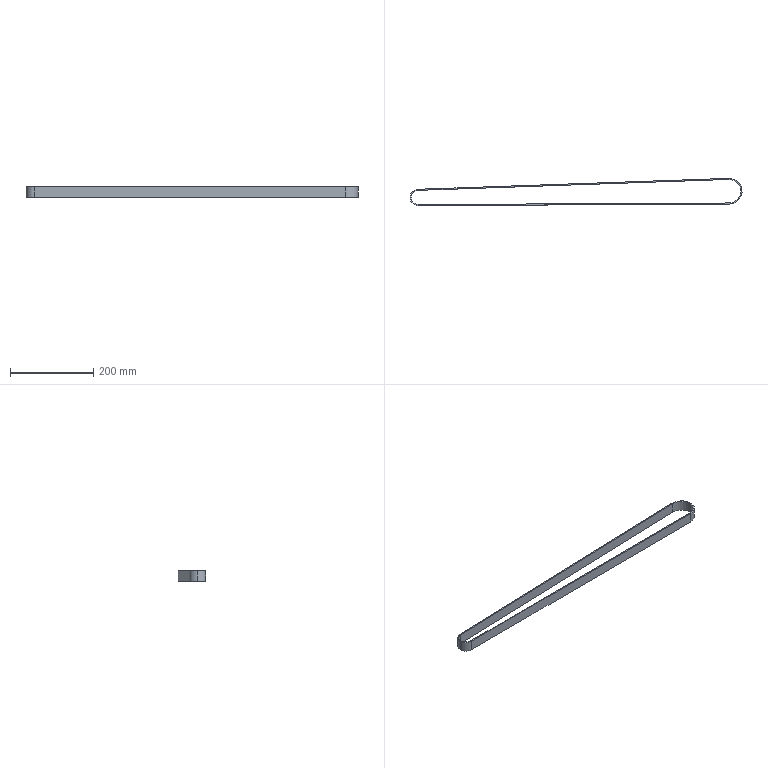Part | STEP file | Belt 4-1^ traction group | 1 solid | 12 faces | box 796.315 x 65.431 x 25 mm | volume 107582 mm3 | cylinder 6 | plane 6 | commonest cylinder face diameters 34 x2 39.24 x2 56.45 x1 61.69 x1
STEP:
#1=CARTESIAN_POINT('',(0.,0.,0.));
#2=DIRECTION('',(0.,0.,1.));
#3=DIRECTION('',(1.,0.,0.));
#4=AXIS2_PLACEMENT_3D('',#1,#2,#3);
#5=CARTESIAN_POINT('',(-0.5968,16.99,25.));
#6=VERTEX_POINT('',#5);
#7=CARTESIAN_POINT('',(-0.5968,16.99,0.));
#8=VERTEX_POINT('',#7);
#9=CARTESIAN_POINT('',(-0.5968,16.99,25.));
#10=DIRECTION('',(0.,0.,-1.));
#11=VECTOR('',#10,1.);
#12=LINE('',#9,#11);
#13=CARTESIAN_POINT('',(0.,0.,25.));
#14=DIRECTION('',(0.,0.,-1.));
#15=DIRECTION('',(-1.,0.,0.));
#16=AXIS2_PLACEMENT_3D('',#13,#14,#15);
#17=CYLINDRICAL_SURFACE('',#16,17.);
#18=CARTESIAN_POINT('',(1.536,0.));
#19=DIRECTION('',(0.,1.));
#20=VECTOR('',#19,1.);
#21=LINE('',#18,#20);
#22=(GEOMETRIC_REPRESENTATION_CONTEXT(2)PARAMETRIC_REPRESENTATION_CONTEXT()REPRESENTATION_CONTEXT('',''));
#23=DEFINITIONAL_REPRESENTATION('',(#21),#22);
#24=PCURVE('',#17,#23);
#25=CARTESIAN_POINT('',(744.859,43.174,25.));
#26=DIRECTION('',(0.0351,-0.9994,0.));
#27=DIRECTION('',(0.9994,0.0351,0.));
#28=AXIS2_PLACEMENT_3D('',#25,#26,#27);
#29=PLANE('',#28);
#30=CARTESIAN_POINT('',(-745.916,0.));
#31=DIRECTION('',(0.,-1.));
#32=VECTOR('',#31,1.);
#33=LINE('',#30,#32);
#34=(GEOMETRIC_REPRESENTATION_CONTEXT(2)PARAMETRIC_REPRESENTATION_CONTEXT()REPRESENTATION_CONTEXT('',''));
#35=DEFINITIONAL_REPRESENTATION('',(#33),#34);
#36=PCURVE('',#29,#35);
#37=SURFACE_CURVE('',#12,(#24,#36),.PCURVE_S1.);
#38=EDGE_CURVE('',#6,#8,#37,.T.);
#39=ORIENTED_EDGE('',*,*,#38,.T.);
#40=CARTESIAN_POINT('',(-17.,0.,0.));
#41=VERTEX_POINT('',#40);
#42=CARTESIAN_POINT('',(0.,0.,0.));
#43=DIRECTION('',(0.,0.,1.));
#44=DIRECTION('',(1.,0.,0.));
#45=AXIS2_PLACEMENT_3D('',#42,#43,#44);
#46=CIRCLE('',#45,17.);
#47=CARTESIAN_POINT('',(3.142,25.));
#48=DIRECTION('',(-1.,0.));
#49=VECTOR('',#48,1.);
#50=LINE('',#47,#49);
#51=(GEOMETRIC_REPRESENTATION_CONTEXT(2)PARAMETRIC_REPRESENTATION_CONTEXT()REPRESENTATION_CONTEXT('',''));
#52=DEFINITIONAL_REPRESENTATION('',(#50),#51);
#53=PCURVE('',#17,#52);
#54=CARTESIAN_POINT('',(745.85,14.966,0.));
#55=DIRECTION('',(0.,0.,1.));
#56=DIRECTION('',(1.,0.,0.));
#57=AXIS2_PLACEMENT_3D('',#54,#55,#56);
#58=PLANE('',#57);
#59=CARTESIAN_POINT('',(-745.85,-14.966));
#60=DIRECTION('',(1.,0.));
#61=AXIS2_PLACEMENT_2D('',#59,#60);
#62=CIRCLE('',#61,17.);
#63=(GEOMETRIC_REPRESENTATION_CONTEXT(2)PARAMETRIC_REPRESENTATION_CONTEXT()REPRESENTATION_CONTEXT('',''));
#64=DEFINITIONAL_REPRESENTATION('',(#62),#63);
#65=PCURVE('',#58,#64);
#66=SURFACE_CURVE('',#46,(#53,#65),.PCURVE_S1.);
#67=EDGE_CURVE('',#8,#41,#66,.T.);
#68=ORIENTED_EDGE('',*,*,#67,.T.);
#69=CARTESIAN_POINT('',(-17.,0.,25.));
#70=VERTEX_POINT('',#69);
#71=CARTESIAN_POINT('',(-17.,0.,25.));
#72=DIRECTION('',(0.,0.,-1.));
#73=VECTOR('',#72,1.);
#74=LINE('',#71,#73);
#75=CARTESIAN_POINT('',(0.,0.));
#76=DIRECTION('',(0.,1.));
#77=VECTOR('',#76,1.);
#78=LINE('',#75,#77);
#79=(GEOMETRIC_REPRESENTATION_CONTEXT(2)PARAMETRIC_REPRESENTATION_CONTEXT()REPRESENTATION_CONTEXT('',''));
#80=DEFINITIONAL_REPRESENTATION('',(#78),#79);
#81=PCURVE('',#17,#80);
#82=CARTESIAN_POINT('',(0.,0.,25.));
#83=DIRECTION('',(0.,0.,-1.));
#84=DIRECTION('',(-1.,0.,0.));
#85=AXIS2_PLACEMENT_3D('',#82,#83,#84);
#86=CYLINDRICAL_SURFACE('',#85,17.);
#87=CARTESIAN_POINT('',(6.283,0.));
#88=DIRECTION('',(0.,1.));
#89=VECTOR('',#88,1.);
#90=LINE('',#87,#89);
#91=(GEOMETRIC_REPRESENTATION_CONTEXT(2)PARAMETRIC_REPRESENTATION_CONTEXT()REPRESENTATION_CONTEXT('',''));
#92=DEFINITIONAL_REPRESENTATION('',(#90),#91);
#93=PCURVE('',#86,#92);
#94=SURFACE_CURVE('',#74,(#81,#93),.PCURVE_S1.);
#95=EDGE_CURVE('',#70,#41,#94,.T.);
#96=ORIENTED_EDGE('',*,*,#95,.F.);
#97=CARTESIAN_POINT('',(0.,0.,25.));
#98=DIRECTION('',(0.,0.,1.));
#99=DIRECTION('',(1.,0.,0.));
#100=AXIS2_PLACEMENT_3D('',#97,#98,#99);
#101=CIRCLE('',#100,17.);
#102=CARTESIAN_POINT('',(3.142,0.));
#103=DIRECTION('',(-1.,0.));
#104=VECTOR('',#103,1.);
#105=LINE('',#102,#104);
#106=(GEOMETRIC_REPRESENTATION_CONTEXT(2)PARAMETRIC_REPRESENTATION_CONTEXT()REPRESENTATION_CONTEXT('',''));
#107=DEFINITIONAL_REPRESENTATION('',(#105),#106);
#108=PCURVE('',#17,#107);
#109=CARTESIAN_POINT('',(745.85,14.966,25.));
#110=DIRECTION('',(0.,0.,1.));
#111=DIRECTION('',(1.,0.,0.));
#112=AXIS2_PLACEMENT_3D('',#109,#110,#111);
#113=PLANE('',#112);
#114=CARTESIAN_POINT('',(-745.85,-14.966));
#115=DIRECTION('',(1.,0.));
#116=AXIS2_PLACEMENT_2D('',#114,#115);
#117=CIRCLE('',#116,17.);
#118=(GEOMETRIC_REPRESENTATION_CONTEXT(2)PARAMETRIC_REPRESENTATION_CONTEXT()REPRESENTATION_CONTEXT('',''));
#119=DEFINITIONAL_REPRESENTATION('',(#117),#118);
#120=PCURVE('',#113,#119);
#121=SURFACE_CURVE('',#101,(#108,#120),.PCURVE_S1.);
#122=EDGE_CURVE('',#6,#70,#121,.T.);
#123=ORIENTED_EDGE('',*,*,#122,.F.);
#124=EDGE_LOOP('',(#39,#68,#96,#123));
#125=FACE_BOUND('',#124,.F.);
#126=ADVANCED_FACE('',(#125),#17,.F.);
#127=CARTESIAN_POINT('',(-19.62,0.,25.));
#128=VERTEX_POINT('',#127);
#129=CARTESIAN_POINT('',(0.09841,-19.62,25.));
#130=VERTEX_POINT('',#129);
#131=CARTESIAN_POINT('',(0.,0.,25.));
#132=DIRECTION('',(0.,0.,1.));
#133=DIRECTION('',(1.,0.,0.));
#134=AXIS2_PLACEMENT_3D('',#131,#132,#133);
#135=CIRCLE('',#134,19.62);
#136=CARTESIAN_POINT('',(0.,0.,25.));
#137=DIRECTION('',(0.,0.,-1.));
#138=DIRECTION('',(-1.,0.,0.));
#139=AXIS2_PLACEMENT_3D('',#136,#137,#138);
#140=CYLINDRICAL_SURFACE('',#139,19.62);
#141=CARTESIAN_POINT('',(9.425,0.));
#142=DIRECTION('',(-1.,0.));
#143=VECTOR('',#142,1.);
#144=LINE('',#141,#143);
#145=(GEOMETRIC_REPRESENTATION_CONTEXT(2)PARAMETRIC_REPRESENTATION_CONTEXT()REPRESENTATION_CONTEXT('',''));
#146=DEFINITIONAL_REPRESENTATION('',(#144),#145);
#147=PCURVE('',#140,#146);
#148=CARTESIAN_POINT('',(-745.85,-14.966));
#149=DIRECTION('',(1.,0.));
#150=AXIS2_PLACEMENT_2D('',#148,#149);
#151=CIRCLE('',#150,19.62);
#152=(GEOMETRIC_REPRESENTATION_CONTEXT(2)PARAMETRIC_REPRESENTATION_CONTEXT()REPRESENTATION_CONTEXT('',''));
#153=DEFINITIONAL_REPRESENTATION('',(#151),#152);
#154=PCURVE('',#113,#153);
#155=SURFACE_CURVE('',#135,(#147,#154),.PCURVE_S1.);
#156=EDGE_CURVE('',#128,#130,#155,.T.);
#157=ORIENTED_EDGE('',*,*,#156,.F.);
#158=CARTESIAN_POINT('',(-19.62,0.,0.));
#159=VERTEX_POINT('',#158);
#160=CARTESIAN_POINT('',(-19.62,0.,25.));
#161=DIRECTION('',(0.,0.,-1.));
#162=VECTOR('',#161,1.);
#163=LINE('',#160,#162);
#164=CARTESIAN_POINT('',(6.283,0.));
#165=DIRECTION('',(0.,1.));
#166=VECTOR('',#165,1.);
#167=LINE('',#164,#166);
#168=(GEOMETRIC_REPRESENTATION_CONTEXT(2)PARAMETRIC_REPRESENTATION_CONTEXT()REPRESENTATION_CONTEXT('',''));
#169=DEFINITIONAL_REPRESENTATION('',(#167),#168);
#170=PCURVE('',#140,#169);
#171=CARTESIAN_POINT('',(0.,0.,25.));
#172=DIRECTION('',(0.,0.,-1.));
#173=DIRECTION('',(-1.,0.,0.));
#174=AXIS2_PLACEMENT_3D('',#171,#172,#173);
#175=CYLINDRICAL_SURFACE('',#174,19.62);
#176=CARTESIAN_POINT('',(0.,0.));
#177=DIRECTION('',(0.,1.));
#178=VECTOR('',#177,1.);
#179=LINE('',#176,#178);
#180=(GEOMETRIC_REPRESENTATION_CONTEXT(2)PARAMETRIC_REPRESENTATION_CONTEXT()REPRESENTATION_CONTEXT('',''));
#181=DEFINITIONAL_REPRESENTATION('',(#179),#180);
#182=PCURVE('',#175,#181);
#183=SURFACE_CURVE('',#163,(#170,#182),.PCURVE_S1.);
#184=EDGE_CURVE('',#128,#159,#183,.T.);
#185=ORIENTED_EDGE('',*,*,#184,.T.);
#186=CARTESIAN_POINT('',(0.09841,-19.62,0.));
#187=VERTEX_POINT('',#186);
#188=CARTESIAN_POINT('',(0.,0.,0.));
#189=DIRECTION('',(0.,0.,1.));
#190=DIRECTION('',(1.,0.,0.));
#191=AXIS2_PLACEMENT_3D('',#188,#189,#190);
#192=CIRCLE('',#191,19.62);
#193=CARTESIAN_POINT('',(9.425,25.));
#194=DIRECTION('',(-1.,0.));
#195=VECTOR('',#194,1.);
#196=LINE('',#193,#195);
#197=(GEOMETRIC_REPRESENTATION_CONTEXT(2)PARAMETRIC_REPRESENTATION_CONTEXT()REPRESENTATION_CONTEXT('',''));
#198=DEFINITIONAL_REPRESENTATION('',(#196),#197);
#199=PCURVE('',#140,#198);
#200=CARTESIAN_POINT('',(-745.85,-14.966));
#201=DIRECTION('',(1.,0.));
#202=AXIS2_PLACEMENT_2D('',#200,#201);
#203=CIRCLE('',#202,19.62);
#204=(GEOMETRIC_REPRESENTATION_CONTEXT(2)PARAMETRIC_REPRESENTATION_CONTEXT()REPRESENTATION_CONTEXT('',''));
#205=DEFINITIONAL_REPRESENTATION('',(#203),#204);
#206=PCURVE('',#58,#205);
#207=SURFACE_CURVE('',#192,(#199,#206),.PCURVE_S1.);
#208=EDGE_CURVE('',#159,#187,#207,.T.);
#209=ORIENTED_EDGE('',*,*,#208,.T.);
#210=CARTESIAN_POINT('',(0.09841,-19.62,25.));
#211=DIRECTION('',(0.,0.,-1.));
#212=VECTOR('',#211,1.);
#213=LINE('',#210,#212);
#214=CARTESIAN_POINT('',(4.707,0.));
#215=DIRECTION('',(0.,1.));
#216=VECTOR('',#215,1.);
#217=LINE('',#214,#216);
#218=(GEOMETRIC_REPRESENTATION_CONTEXT(2)PARAMETRIC_REPRESENTATION_CONTEXT()REPRESENTATION_CONTEXT('',''));
#219=DEFINITIONAL_REPRESENTATION('',(#217),#218);
#220=PCURVE('',#140,#219);
#221=CARTESIAN_POINT('',(0.09841,-19.62,25.));
#222=DIRECTION('',(-0.005016,1.,0.));
#223=DIRECTION('',(-1.,-0.005016,0.));
#224=AXIS2_PLACEMENT_3D('',#221,#222,#223);
#225=PLANE('',#224);
#226=CARTESIAN_POINT('',(0.,0.));
#227=DIRECTION('',(0.,-1.));
#228=VECTOR('',#227,1.);
#229=LINE('',#226,#228);
#230=(GEOMETRIC_REPRESENTATION_CONTEXT(2)PARAMETRIC_REPRESENTATION_CONTEXT()REPRESENTATION_CONTEXT('',''));
#231=DEFINITIONAL_REPRESENTATION('',(#229),#230);
#232=PCURVE('',#225,#231);
#233=SURFACE_CURVE('',#213,(#220,#232),.PCURVE_S1.);
#234=EDGE_CURVE('',#130,#187,#233,.T.);
#235=ORIENTED_EDGE('',*,*,#234,.F.);
#236=EDGE_LOOP('',(#157,#185,#209,#235));
#237=FACE_BOUND('',#236,.T.);
#238=ADVANCED_FACE('',(#237),#140,.T.);
#239=CARTESIAN_POINT('',(746.005,-15.878,25.));
#240=VERTEX_POINT('',#239);
#241=CARTESIAN_POINT('',(744.767,45.792,25.));
#242=VERTEX_POINT('',#241);
#243=CARTESIAN_POINT('',(745.85,14.966,25.));
#244=DIRECTION('',(0.,0.,1.));
#245=DIRECTION('',(1.,0.,0.));
#246=AXIS2_PLACEMENT_3D('',#243,#244,#245);
#247=CIRCLE('',#246,30.845);
#248=CARTESIAN_POINT('',(0.,0.));
#249=DIRECTION('',(1.,0.));
#250=AXIS2_PLACEMENT_2D('',#248,#249);
#251=CIRCLE('',#250,30.845);
#252=(GEOMETRIC_REPRESENTATION_CONTEXT(2)PARAMETRIC_REPRESENTATION_CONTEXT()REPRESENTATION_CONTEXT('',''));
#253=DEFINITIONAL_REPRESENTATION('',(#251),#252);
#254=PCURVE('',#113,#253);
#255=CARTESIAN_POINT('',(745.85,14.966,25.));
#256=DIRECTION('',(0.,0.,-1.));
#257=DIRECTION('',(-1.,0.,0.));
#258=AXIS2_PLACEMENT_3D('',#255,#256,#257);
#259=CYLINDRICAL_SURFACE('',#258,30.845);
#260=CARTESIAN_POINT('',(9.425,0.));
#261=DIRECTION('',(-1.,0.));
#262=VECTOR('',#261,1.);
#263=LINE('',#260,#262);
#264=(GEOMETRIC_REPRESENTATION_CONTEXT(2)PARAMETRIC_REPRESENTATION_CONTEXT()REPRESENTATION_CONTEXT('',''));
#265=DEFINITIONAL_REPRESENTATION('',(#263),#264);
#266=PCURVE('',#259,#265);
#267=SURFACE_CURVE('',#247,(#254,#266),.PCURVE_S1.);
#268=EDGE_CURVE('',#240,#242,#267,.T.);
#269=ORIENTED_EDGE('',*,*,#268,.T.);
#270=CARTESIAN_POINT('',(-0.6887,19.608,25.));
#271=VERTEX_POINT('',#270);
#272=CARTESIAN_POINT('',(744.767,45.792,25.));
#273=DIRECTION('',(-0.9994,-0.0351,0.));
#274=VECTOR('',#273,1.);
#275=LINE('',#272,#274);
#276=CARTESIAN_POINT('',(-1.083,30.826));
#277=DIRECTION('',(-0.9994,-0.0351));
#278=VECTOR('',#277,1.);
#279=LINE('',#276,#278);
#280=(GEOMETRIC_REPRESENTATION_CONTEXT(2)PARAMETRIC_REPRESENTATION_CONTEXT()REPRESENTATION_CONTEXT('',''));
#281=DEFINITIONAL_REPRESENTATION('',(#279),#280);
#282=PCURVE('',#113,#281);
#283=CARTESIAN_POINT('',(744.767,45.792,25.));
#284=DIRECTION('',(0.0351,-0.9994,0.));
#285=DIRECTION('',(0.9994,0.0351,0.));
#286=AXIS2_PLACEMENT_3D('',#283,#284,#285);
#287=PLANE('',#286);
#288=CARTESIAN_POINT('',(0.,0.));
#289=DIRECTION('',(-1.,0.));
#290=VECTOR('',#289,1.);
#291=LINE('',#288,#290);
#292=(GEOMETRIC_REPRESENTATION_CONTEXT(2)PARAMETRIC_REPRESENTATION_CONTEXT()REPRESENTATION_CONTEXT('',''));
#293=DEFINITIONAL_REPRESENTATION('',(#291),#292);
#294=PCURVE('',#287,#293);
#295=SURFACE_CURVE('',#275,(#282,#294),.PCURVE_S1.);
#296=EDGE_CURVE('',#242,#271,#295,.T.);
#297=ORIENTED_EDGE('',*,*,#296,.T.);
#298=CARTESIAN_POINT('',(0.,0.,25.));
#299=DIRECTION('',(0.,0.,1.));
#300=DIRECTION('',(1.,0.,0.));
#301=AXIS2_PLACEMENT_3D('',#298,#299,#300);
#302=CIRCLE('',#301,19.62);
#303=CARTESIAN_POINT('',(-745.85,-14.966));
#304=DIRECTION('',(1.,0.));
#305=AXIS2_PLACEMENT_2D('',#303,#304);
#306=CIRCLE('',#305,19.62);
#307=(GEOMETRIC_REPRESENTATION_CONTEXT(2)PARAMETRIC_REPRESENTATION_CONTEXT()REPRESENTATION_CONTEXT('',''));
#308=DEFINITIONAL_REPRESENTATION('',(#306),#307);
#309=PCURVE('',#113,#308);
#310=CARTESIAN_POINT('',(3.142,0.));
#311=DIRECTION('',(-1.,0.));
#312=VECTOR('',#311,1.);
#313=LINE('',#310,#312);
#314=(GEOMETRIC_REPRESENTATION_CONTEXT(2)PARAMETRIC_REPRESENTATION_CONTEXT()REPRESENTATION_CONTEXT('',''));
#315=DEFINITIONAL_REPRESENTATION('',(#313),#314);
#316=PCURVE('',#175,#315);
#317=SURFACE_CURVE('',#302,(#309,#316),.PCURVE_S1.);
#318=EDGE_CURVE('',#271,#128,#317,.T.);
#319=ORIENTED_EDGE('',*,*,#318,.T.);
#320=ORIENTED_EDGE('',*,*,#156,.T.);
#321=CARTESIAN_POINT('',(0.09841,-19.62,25.));
#322=DIRECTION('',(1.,0.005016,0.));
#323=VECTOR('',#322,1.);
#324=LINE('',#321,#323);
#325=CARTESIAN_POINT('',(-745.751,-34.586));
#326=DIRECTION('',(1.,0.005016));
#327=VECTOR('',#326,1.);
#328=LINE('',#325,#327);
#329=(GEOMETRIC_REPRESENTATION_CONTEXT(2)PARAMETRIC_REPRESENTATION_CONTEXT()REPRESENTATION_CONTEXT('',''));
#330=DEFINITIONAL_REPRESENTATION('',(#328),#329);
#331=PCURVE('',#113,#330);
#332=CARTESIAN_POINT('',(0.,0.));
#333=DIRECTION('',(-1.,0.));
#334=VECTOR('',#333,1.);
#335=LINE('',#332,#334);
#336=(GEOMETRIC_REPRESENTATION_CONTEXT(2)PARAMETRIC_REPRESENTATION_CONTEXT()REPRESENTATION_CONTEXT('',''));
#337=DEFINITIONAL_REPRESENTATION('',(#335),#336);
#338=PCURVE('',#225,#337);
#339=SURFACE_CURVE('',#324,(#331,#338),.PCURVE_S1.);
#340=EDGE_CURVE('',#130,#240,#339,.T.);
#341=ORIENTED_EDGE('',*,*,#340,.T.);
#342=EDGE_LOOP('',(#269,#297,#319,#320,#341));
#343=FACE_BOUND('',#342,.T.);
#344=CARTESIAN_POINT('',(744.859,43.174,25.));
#345=VERTEX_POINT('',#344);
#346=CARTESIAN_POINT('',(744.859,43.174,25.));
#347=DIRECTION('',(-0.9994,-0.0351,0.));
#348=VECTOR('',#347,1.);
#349=LINE('',#346,#348);
#350=CARTESIAN_POINT('',(-0.9908,28.208));
#351=DIRECTION('',(-0.9994,-0.0351));
#352=VECTOR('',#351,1.);
#353=LINE('',#350,#352);
#354=(GEOMETRIC_REPRESENTATION_CONTEXT(2)PARAMETRIC_REPRESENTATION_CONTEXT()REPRESENTATION_CONTEXT('',''));
#355=DEFINITIONAL_REPRESENTATION('',(#353),#354);
#356=PCURVE('',#113,#355);
#357=CARTESIAN_POINT('',(0.,0.));
#358=DIRECTION('',(-1.,0.));
#359=VECTOR('',#358,1.);
#360=LINE('',#357,#359);
#361=(GEOMETRIC_REPRESENTATION_CONTEXT(2)PARAMETRIC_REPRESENTATION_CONTEXT()REPRESENTATION_CONTEXT('',''));
#362=DEFINITIONAL_REPRESENTATION('',(#360),#361);
#363=PCURVE('',#29,#362);
#364=SURFACE_CURVE('',#349,(#356,#363),.PCURVE_S1.);
#365=EDGE_CURVE('',#345,#6,#364,.T.);
#366=ORIENTED_EDGE('',*,*,#365,.F.);
#367=CARTESIAN_POINT('',(745.991,-13.258,25.));
#368=VERTEX_POINT('',#367);
#369=CARTESIAN_POINT('',(745.85,14.966,25.));
#370=DIRECTION('',(0.,0.,1.));
#371=DIRECTION('',(1.,0.,0.));
#372=AXIS2_PLACEMENT_3D('',#369,#370,#371);
#373=CIRCLE('',#372,28.225);
#374=CARTESIAN_POINT('',(0.,0.));
#375=DIRECTION('',(1.,0.));
#376=AXIS2_PLACEMENT_2D('',#374,#375);
#377=CIRCLE('',#376,28.225);
#378=(GEOMETRIC_REPRESENTATION_CONTEXT(2)PARAMETRIC_REPRESENTATION_CONTEXT()REPRESENTATION_CONTEXT('',''));
#379=DEFINITIONAL_REPRESENTATION('',(#377),#378);
#380=PCURVE('',#113,#379);
#381=CARTESIAN_POINT('',(745.85,14.966,25.));
#382=DIRECTION('',(0.,0.,-1.));
#383=DIRECTION('',(-1.,0.,0.));
#384=AXIS2_PLACEMENT_3D('',#381,#382,#383);
#385=CYLINDRICAL_SURFACE('',#384,28.225);
#386=CARTESIAN_POINT('',(9.425,0.));
#387=DIRECTION('',(-1.,0.));
#388=VECTOR('',#387,1.);
#389=LINE('',#386,#388);
#390=(GEOMETRIC_REPRESENTATION_CONTEXT(2)PARAMETRIC_REPRESENTATION_CONTEXT()REPRESENTATION_CONTEXT('',''));
#391=DEFINITIONAL_REPRESENTATION('',(#389),#390);
#392=PCURVE('',#385,#391);
#393=SURFACE_CURVE('',#373,(#380,#392),.PCURVE_S1.);
#394=EDGE_CURVE('',#368,#345,#393,.T.);
#395=ORIENTED_EDGE('',*,*,#394,.F.);
#396=CARTESIAN_POINT('',(0.08527,-17.,25.));
#397=VERTEX_POINT('',#396);
#398=CARTESIAN_POINT('',(0.08527,-17.,25.));
#399=DIRECTION('',(1.,0.005016,0.));
#400=VECTOR('',#399,1.);
#401=LINE('',#398,#400);
#402=CARTESIAN_POINT('',(-745.765,-31.966));
#403=DIRECTION('',(1.,0.005016));
#404=VECTOR('',#403,1.);
#405=LINE('',#402,#404);
#406=(GEOMETRIC_REPRESENTATION_CONTEXT(2)PARAMETRIC_REPRESENTATION_CONTEXT()REPRESENTATION_CONTEXT('',''));
#407=DEFINITIONAL_REPRESENTATION('',(#405),#406);
#408=PCURVE('',#113,#407);
#409=CARTESIAN_POINT('',(0.08527,-17.,25.));
#410=DIRECTION('',(-0.005016,1.,0.));
#411=DIRECTION('',(-1.,-0.005016,0.));
#412=AXIS2_PLACEMENT_3D('',#409,#410,#411);
#413=PLANE('',#412);
#414=CARTESIAN_POINT('',(0.,0.));
#415=DIRECTION('',(-1.,0.));
#416=VECTOR('',#415,1.);
#417=LINE('',#414,#416);
#418=(GEOMETRIC_REPRESENTATION_CONTEXT(2)PARAMETRIC_REPRESENTATION_CONTEXT()REPRESENTATION_CONTEXT('',''));
#419=DEFINITIONAL_REPRESENTATION('',(#417),#418);
#420=PCURVE('',#413,#419);
#421=SURFACE_CURVE('',#401,(#408,#420),.PCURVE_S1.);
#422=EDGE_CURVE('',#397,#368,#421,.T.);
#423=ORIENTED_EDGE('',*,*,#422,.F.);
#424=CARTESIAN_POINT('',(0.,0.,25.));
#425=DIRECTION('',(0.,0.,1.));
#426=DIRECTION('',(1.,0.,0.));
#427=AXIS2_PLACEMENT_3D('',#424,#425,#426);
#428=CIRCLE('',#427,17.);
#429=CARTESIAN_POINT('',(-745.85,-14.966));
#430=DIRECTION('',(1.,0.));
#431=AXIS2_PLACEMENT_2D('',#429,#430);
#432=CIRCLE('',#431,17.);
#433=(GEOMETRIC_REPRESENTATION_CONTEXT(2)PARAMETRIC_REPRESENTATION_CONTEXT()REPRESENTATION_CONTEXT('',''));
#434=DEFINITIONAL_REPRESENTATION('',(#432),#433);
#435=PCURVE('',#113,#434);
#436=CARTESIAN_POINT('',(9.425,0.));
#437=DIRECTION('',(-1.,0.));
#438=VECTOR('',#437,1.);
#439=LINE('',#436,#438);
#440=(GEOMETRIC_REPRESENTATION_CONTEXT(2)PARAMETRIC_REPRESENTATION_CONTEXT()REPRESENTATION_CONTEXT('',''));
#441=DEFINITIONAL_REPRESENTATION('',(#439),#440);
#442=PCURVE('',#86,#441);
#443=SURFACE_CURVE('',#428,(#435,#442),.PCURVE_S1.);
#444=EDGE_CURVE('',#70,#397,#443,.T.);
#445=ORIENTED_EDGE('',*,*,#444,.F.);
#446=ORIENTED_EDGE('',*,*,#122,.F.);
#447=EDGE_LOOP('',(#366,#395,#423,#445,#446));
#448=FACE_BOUND('',#447,.T.);
#449=ADVANCED_FACE('',(#343,#448),#113,.T.);
#450=CARTESIAN_POINT('',(746.005,-15.878,0.));
#451=VERTEX_POINT('',#450);
#452=CARTESIAN_POINT('',(744.767,45.792,0.));
#453=VERTEX_POINT('',#452);
#454=CARTESIAN_POINT('',(745.85,14.966,0.));
#455=DIRECTION('',(0.,0.,1.));
#456=DIRECTION('',(1.,0.,0.));
#457=AXIS2_PLACEMENT_3D('',#454,#455,#456);
#458=CIRCLE('',#457,30.845);
#459=CARTESIAN_POINT('',(0.,0.));
#460=DIRECTION('',(1.,0.));
#461=AXIS2_PLACEMENT_2D('',#459,#460);
#462=CIRCLE('',#461,30.845);
#463=(GEOMETRIC_REPRESENTATION_CONTEXT(2)PARAMETRIC_REPRESENTATION_CONTEXT()REPRESENTATION_CONTEXT('',''));
#464=DEFINITIONAL_REPRESENTATION('',(#462),#463);
#465=PCURVE('',#58,#464);
#466=CARTESIAN_POINT('',(9.425,25.));
#467=DIRECTION('',(-1.,0.));
#468=VECTOR('',#467,1.);
#469=LINE('',#466,#468);
#470=(GEOMETRIC_REPRESENTATION_CONTEXT(2)PARAMETRIC_REPRESENTATION_CONTEXT()REPRESENTATION_CONTEXT('',''));
#471=DEFINITIONAL_REPRESENTATION('',(#469),#470);
#472=PCURVE('',#259,#471);
#473=SURFACE_CURVE('',#458,(#465,#472),.PCURVE_S1.);
#474=EDGE_CURVE('',#451,#453,#473,.T.);
#475=ORIENTED_EDGE('',*,*,#474,.F.);
#476=CARTESIAN_POINT('',(0.09841,-19.62,0.));
#477=DIRECTION('',(1.,0.005016,0.));
#478=VECTOR('',#477,1.);
#479=LINE('',#476,#478);
#480=CARTESIAN_POINT('',(-745.751,-34.586));
#481=DIRECTION('',(1.,0.005016));
#482=VECTOR('',#481,1.);
#483=LINE('',#480,#482);
#484=(GEOMETRIC_REPRESENTATION_CONTEXT(2)PARAMETRIC_REPRESENTATION_CONTEXT()REPRESENTATION_CONTEXT('',''));
#485=DEFINITIONAL_REPRESENTATION('',(#483),#484);
#486=PCURVE('',#58,#485);
#487=CARTESIAN_POINT('',(0.,-25.));
#488=DIRECTION('',(-1.,0.));
#489=VECTOR('',#488,1.);
#490=LINE('',#487,#489);
#491=(GEOMETRIC_REPRESENTATION_CONTEXT(2)PARAMETRIC_REPRESENTATION_CONTEXT()REPRESENTATION_CONTEXT('',''));
#492=DEFINITIONAL_REPRESENTATION('',(#490),#491);
#493=PCURVE('',#225,#492);
#494=SURFACE_CURVE('',#479,(#486,#493),.PCURVE_S1.);
#495=EDGE_CURVE('',#187,#451,#494,.T.);
#496=ORIENTED_EDGE('',*,*,#495,.F.);
#497=ORIENTED_EDGE('',*,*,#208,.F.);
#498=CARTESIAN_POINT('',(-0.6887,19.608,0.));
#499=VERTEX_POINT('',#498);
#500=CARTESIAN_POINT('',(0.,0.,0.));
#501=DIRECTION('',(0.,0.,1.));
#502=DIRECTION('',(1.,0.,0.));
#503=AXIS2_PLACEMENT_3D('',#500,#501,#502);
#504=CIRCLE('',#503,19.62);
#505=CARTESIAN_POINT('',(-745.85,-14.966));
#506=DIRECTION('',(1.,0.));
#507=AXIS2_PLACEMENT_2D('',#505,#506);
#508=CIRCLE('',#507,19.62);
#509=(GEOMETRIC_REPRESENTATION_CONTEXT(2)PARAMETRIC_REPRESENTATION_CONTEXT()REPRESENTATION_CONTEXT('',''));
#510=DEFINITIONAL_REPRESENTATION('',(#508),#509);
#511=PCURVE('',#58,#510);
#512=CARTESIAN_POINT('',(3.142,25.));
#513=DIRECTION('',(-1.,0.));
#514=VECTOR('',#513,1.);
#515=LINE('',#512,#514);
#516=(GEOMETRIC_REPRESENTATION_CONTEXT(2)PARAMETRIC_REPRESENTATION_CONTEXT()REPRESENTATION_CONTEXT('',''));
#517=DEFINITIONAL_REPRESENTATION('',(#515),#516);
#518=PCURVE('',#175,#517);
#519=SURFACE_CURVE('',#504,(#511,#518),.PCURVE_S1.);
#520=EDGE_CURVE('',#499,#159,#519,.T.);
#521=ORIENTED_EDGE('',*,*,#520,.F.);
#522=CARTESIAN_POINT('',(744.767,45.792,0.));
#523=DIRECTION('',(-0.9994,-0.0351,0.));
#524=VECTOR('',#523,1.);
#525=LINE('',#522,#524);
#526=CARTESIAN_POINT('',(-1.083,30.826));
#527=DIRECTION('',(-0.9994,-0.0351));
#528=VECTOR('',#527,1.);
#529=LINE('',#526,#528);
#530=(GEOMETRIC_REPRESENTATION_CONTEXT(2)PARAMETRIC_REPRESENTATION_CONTEXT()REPRESENTATION_CONTEXT('',''));
#531=DEFINITIONAL_REPRESENTATION('',(#529),#530);
#532=PCURVE('',#58,#531);
#533=CARTESIAN_POINT('',(0.,-25.));
#534=DIRECTION('',(-1.,0.));
#535=VECTOR('',#534,1.);
#536=LINE('',#533,#535);
#537=(GEOMETRIC_REPRESENTATION_CONTEXT(2)PARAMETRIC_REPRESENTATION_CONTEXT()REPRESENTATION_CONTEXT('',''));
#538=DEFINITIONAL_REPRESENTATION('',(#536),#537);
#539=PCURVE('',#287,#538);
#540=SURFACE_CURVE('',#525,(#532,#539),.PCURVE_S1.);
#541=EDGE_CURVE('',#453,#499,#540,.T.);
#542=ORIENTED_EDGE('',*,*,#541,.F.);
#543=EDGE_LOOP('',(#475,#496,#497,#521,#542));
#544=FACE_BOUND('',#543,.T.);
#545=CARTESIAN_POINT('',(745.991,-13.258,0.));
#546=VERTEX_POINT('',#545);
#547=CARTESIAN_POINT('',(744.859,43.174,0.));
#548=VERTEX_POINT('',#547);
#549=CARTESIAN_POINT('',(745.85,14.966,0.));
#550=DIRECTION('',(0.,0.,1.));
#551=DIRECTION('',(1.,0.,0.));
#552=AXIS2_PLACEMENT_3D('',#549,#550,#551);
#553=CIRCLE('',#552,28.225);
#554=CARTESIAN_POINT('',(0.,0.));
#555=DIRECTION('',(1.,0.));
#556=AXIS2_PLACEMENT_2D('',#554,#555);
#557=CIRCLE('',#556,28.225);
#558=(GEOMETRIC_REPRESENTATION_CONTEXT(2)PARAMETRIC_REPRESENTATION_CONTEXT()REPRESENTATION_CONTEXT('',''));
#559=DEFINITIONAL_REPRESENTATION('',(#557),#558);
#560=PCURVE('',#58,#559);
#561=CARTESIAN_POINT('',(9.425,25.));
#562=DIRECTION('',(-1.,0.));
#563=VECTOR('',#562,1.);
#564=LINE('',#561,#563);
#565=(GEOMETRIC_REPRESENTATION_CONTEXT(2)PARAMETRIC_REPRESENTATION_CONTEXT()REPRESENTATION_CONTEXT('',''));
#566=DEFINITIONAL_REPRESENTATION('',(#564),#565);
#567=PCURVE('',#385,#566);
#568=SURFACE_CURVE('',#553,(#560,#567),.PCURVE_S1.);
#569=EDGE_CURVE('',#546,#548,#568,.T.);
#570=ORIENTED_EDGE('',*,*,#569,.T.);
#571=CARTESIAN_POINT('',(744.859,43.174,0.));
#572=DIRECTION('',(-0.9994,-0.0351,0.));
#573=VECTOR('',#572,1.);
#574=LINE('',#571,#573);
#575=CARTESIAN_POINT('',(-0.9908,28.208));
#576=DIRECTION('',(-0.9994,-0.0351));
#577=VECTOR('',#576,1.);
#578=LINE('',#575,#577);
#579=(GEOMETRIC_REPRESENTATION_CONTEXT(2)PARAMETRIC_REPRESENTATION_CONTEXT()REPRESENTATION_CONTEXT('',''));
#580=DEFINITIONAL_REPRESENTATION('',(#578),#579);
#581=PCURVE('',#58,#580);
#582=CARTESIAN_POINT('',(0.,-25.));
#583=DIRECTION('',(-1.,0.));
#584=VECTOR('',#583,1.);
#585=LINE('',#582,#584);
#586=(GEOMETRIC_REPRESENTATION_CONTEXT(2)PARAMETRIC_REPRESENTATION_CONTEXT()REPRESENTATION_CONTEXT('',''));
#587=DEFINITIONAL_REPRESENTATION('',(#585),#586);
#588=PCURVE('',#29,#587);
#589=SURFACE_CURVE('',#574,(#581,#588),.PCURVE_S1.);
#590=EDGE_CURVE('',#548,#8,#589,.T.);
#591=ORIENTED_EDGE('',*,*,#590,.T.);
#592=ORIENTED_EDGE('',*,*,#67,.T.);
#593=CARTESIAN_POINT('',(0.08527,-17.,0.));
#594=VERTEX_POINT('',#593);
#595=CARTESIAN_POINT('',(0.,0.,0.));
#596=DIRECTION('',(0.,0.,1.));
#597=DIRECTION('',(1.,0.,0.));
#598=AXIS2_PLACEMENT_3D('',#595,#596,#597);
#599=CIRCLE('',#598,17.);
#600=CARTESIAN_POINT('',(-745.85,-14.966));
#601=DIRECTION('',(1.,0.));
#602=AXIS2_PLACEMENT_2D('',#600,#601);
#603=CIRCLE('',#602,17.);
#604=(GEOMETRIC_REPRESENTATION_CONTEXT(2)PARAMETRIC_REPRESENTATION_CONTEXT()REPRESENTATION_CONTEXT('',''));
#605=DEFINITIONAL_REPRESENTATION('',(#603),#604);
#606=PCURVE('',#58,#605);
#607=CARTESIAN_POINT('',(9.425,25.));
#608=DIRECTION('',(-1.,0.));
#609=VECTOR('',#608,1.);
#610=LINE('',#607,#609);
#611=(GEOMETRIC_REPRESENTATION_CONTEXT(2)PARAMETRIC_REPRESENTATION_CONTEXT()REPRESENTATION_CONTEXT('',''));
#612=DEFINITIONAL_REPRESENTATION('',(#610),#611);
#613=PCURVE('',#86,#612);
#614=SURFACE_CURVE('',#599,(#606,#613),.PCURVE_S1.);
#615=EDGE_CURVE('',#41,#594,#614,.T.);
#616=ORIENTED_EDGE('',*,*,#615,.T.);
#617=CARTESIAN_POINT('',(0.08527,-17.,0.));
#618=DIRECTION('',(1.,0.005016,0.));
#619=VECTOR('',#618,1.);
#620=LINE('',#617,#619);
#621=CARTESIAN_POINT('',(-745.765,-31.966));
#622=DIRECTION('',(1.,0.005016));
#623=VECTOR('',#622,1.);
#624=LINE('',#621,#623);
#625=(GEOMETRIC_REPRESENTATION_CONTEXT(2)PARAMETRIC_REPRESENTATION_CONTEXT()REPRESENTATION_CONTEXT('',''));
#626=DEFINITIONAL_REPRESENTATION('',(#624),#625);
#627=PCURVE('',#58,#626);
#628=CARTESIAN_POINT('',(0.,-25.));
#629=DIRECTION('',(-1.,0.));
#630=VECTOR('',#629,1.);
#631=LINE('',#628,#630);
#632=(GEOMETRIC_REPRESENTATION_CONTEXT(2)PARAMETRIC_REPRESENTATION_CONTEXT()REPRESENTATION_CONTEXT('',''));
#633=DEFINITIONAL_REPRESENTATION('',(#631),#632);
#634=PCURVE('',#413,#633);
#635=SURFACE_CURVE('',#620,(#627,#634),.PCURVE_S1.);
#636=EDGE_CURVE('',#594,#546,#635,.T.);
#637=ORIENTED_EDGE('',*,*,#636,.T.);
#638=EDGE_LOOP('',(#570,#591,#592,#616,#637));
#639=FACE_BOUND('',#638,.T.);
#640=ADVANCED_FACE('',(#544,#639),#58,.F.);
#641=ORIENTED_EDGE('',*,*,#474,.T.);
#642=CARTESIAN_POINT('',(744.767,45.792,25.));
#643=DIRECTION('',(0.,0.,-1.));
#644=VECTOR('',#643,1.);
#645=LINE('',#642,#644);
#646=CARTESIAN_POINT('',(1.536,0.));
#647=DIRECTION('',(0.,1.));
#648=VECTOR('',#647,1.);
#649=LINE('',#646,#648);
#650=(GEOMETRIC_REPRESENTATION_CONTEXT(2)PARAMETRIC_REPRESENTATION_CONTEXT()REPRESENTATION_CONTEXT('',''));
#651=DEFINITIONAL_REPRESENTATION('',(#649),#650);
#652=PCURVE('',#259,#651);
#653=CARTESIAN_POINT('',(0.,0.));
#654=DIRECTION('',(0.,-1.));
#655=VECTOR('',#654,1.);
#656=LINE('',#653,#655);
#657=(GEOMETRIC_REPRESENTATION_CONTEXT(2)PARAMETRIC_REPRESENTATION_CONTEXT()REPRESENTATION_CONTEXT('',''));
#658=DEFINITIONAL_REPRESENTATION('',(#656),#657);
#659=PCURVE('',#287,#658);
#660=SURFACE_CURVE('',#645,(#652,#659),.PCURVE_S1.);
#661=EDGE_CURVE('',#242,#453,#660,.T.);
#662=ORIENTED_EDGE('',*,*,#661,.F.);
#663=ORIENTED_EDGE('',*,*,#268,.F.);
#664=CARTESIAN_POINT('',(746.005,-15.878,25.));
#665=DIRECTION('',(0.,0.,-1.));
#666=VECTOR('',#665,1.);
#667=LINE('',#664,#666);
#668=CARTESIAN_POINT('',(4.707,0.));
#669=DIRECTION('',(0.,1.));
#670=VECTOR('',#669,1.);
#671=LINE('',#668,#670);
#672=(GEOMETRIC_REPRESENTATION_CONTEXT(2)PARAMETRIC_REPRESENTATION_CONTEXT()REPRESENTATION_CONTEXT('',''));
#673=DEFINITIONAL_REPRESENTATION('',(#671),#672);
#674=PCURVE('',#259,#673);
#675=CARTESIAN_POINT('',(-745.916,0.));
#676=DIRECTION('',(0.,-1.));
#677=VECTOR('',#676,1.);
#678=LINE('',#675,#677);
#679=(GEOMETRIC_REPRESENTATION_CONTEXT(2)PARAMETRIC_REPRESENTATION_CONTEXT()REPRESENTATION_CONTEXT('',''));
#680=DEFINITIONAL_REPRESENTATION('',(#678),#679);
#681=PCURVE('',#225,#680);
#682=SURFACE_CURVE('',#667,(#674,#681),.PCURVE_S1.);
#683=EDGE_CURVE('',#240,#451,#682,.T.);
#684=ORIENTED_EDGE('',*,*,#683,.T.);
#685=EDGE_LOOP('',(#641,#662,#663,#684));
#686=FACE_BOUND('',#685,.T.);
#687=ADVANCED_FACE('',(#686),#259,.T.);
#688=ORIENTED_EDGE('',*,*,#541,.T.);
#689=CARTESIAN_POINT('',(-0.6887,19.608,25.));
#690=DIRECTION('',(0.,0.,-1.));
#691=VECTOR('',#690,1.);
#692=LINE('',#689,#691);
#693=CARTESIAN_POINT('',(-745.916,0.));
#694=DIRECTION('',(0.,-1.));
#695=VECTOR('',#694,1.);
#696=LINE('',#693,#695);
#697=(GEOMETRIC_REPRESENTATION_CONTEXT(2)PARAMETRIC_REPRESENTATION_CONTEXT()REPRESENTATION_CONTEXT('',''));
#698=DEFINITIONAL_REPRESENTATION('',(#696),#697);
#699=PCURVE('',#287,#698);
#700=CARTESIAN_POINT('',(1.536,0.));
#701=DIRECTION('',(0.,1.));
#702=VECTOR('',#701,1.);
#703=LINE('',#700,#702);
#704=(GEOMETRIC_REPRESENTATION_CONTEXT(2)PARAMETRIC_REPRESENTATION_CONTEXT()REPRESENTATION_CONTEXT('',''));
#705=DEFINITIONAL_REPRESENTATION('',(#703),#704);
#706=PCURVE('',#175,#705);
#707=SURFACE_CURVE('',#692,(#699,#706),.PCURVE_S1.);
#708=EDGE_CURVE('',#271,#499,#707,.T.);
#709=ORIENTED_EDGE('',*,*,#708,.F.);
#710=ORIENTED_EDGE('',*,*,#296,.F.);
#711=ORIENTED_EDGE('',*,*,#661,.T.);
#712=EDGE_LOOP('',(#688,#709,#710,#711));
#713=FACE_BOUND('',#712,.T.);
#714=ADVANCED_FACE('',(#713),#287,.F.);
#715=ORIENTED_EDGE('',*,*,#184,.F.);
#716=ORIENTED_EDGE('',*,*,#318,.F.);
#717=ORIENTED_EDGE('',*,*,#708,.T.);
#718=ORIENTED_EDGE('',*,*,#520,.T.);
#719=EDGE_LOOP('',(#715,#716,#717,#718));
#720=FACE_BOUND('',#719,.T.);
#721=ADVANCED_FACE('',(#720),#175,.T.);
#722=ORIENTED_EDGE('',*,*,#495,.T.);
#723=ORIENTED_EDGE('',*,*,#683,.F.);
#724=ORIENTED_EDGE('',*,*,#340,.F.);
#725=ORIENTED_EDGE('',*,*,#234,.T.);
#726=EDGE_LOOP('',(#722,#723,#724,#725));
#727=FACE_BOUND('',#726,.T.);
#728=ADVANCED_FACE('',(#727),#225,.F.);
#729=CARTESIAN_POINT('',(744.859,43.174,25.));
#730=DIRECTION('',(0.,0.,-1.));
#731=VECTOR('',#730,1.);
#732=LINE('',#729,#731);
#733=CARTESIAN_POINT('',(1.536,0.));
#734=DIRECTION('',(0.,1.));
#735=VECTOR('',#734,1.);
#736=LINE('',#733,#735);
#737=(GEOMETRIC_REPRESENTATION_CONTEXT(2)PARAMETRIC_REPRESENTATION_CONTEXT()REPRESENTATION_CONTEXT('',''));
#738=DEFINITIONAL_REPRESENTATION('',(#736),#737);
#739=PCURVE('',#385,#738);
#740=CARTESIAN_POINT('',(0.,0.));
#741=DIRECTION('',(0.,-1.));
#742=VECTOR('',#741,1.);
#743=LINE('',#740,#742);
#744=(GEOMETRIC_REPRESENTATION_CONTEXT(2)PARAMETRIC_REPRESENTATION_CONTEXT()REPRESENTATION_CONTEXT('',''));
#745=DEFINITIONAL_REPRESENTATION('',(#743),#744);
#746=PCURVE('',#29,#745);
#747=SURFACE_CURVE('',#732,(#739,#746),.PCURVE_S1.);
#748=EDGE_CURVE('',#345,#548,#747,.T.);
#749=ORIENTED_EDGE('',*,*,#748,.F.);
#750=ORIENTED_EDGE('',*,*,#394,.F.);
#751=CARTESIAN_POINT('',(745.991,-13.258,25.));
#752=DIRECTION('',(0.,0.,-1.));
#753=VECTOR('',#752,1.);
#754=LINE('',#751,#753);
#755=CARTESIAN_POINT('',(4.707,0.));
#756=DIRECTION('',(0.,1.));
#757=VECTOR('',#756,1.);
#758=LINE('',#755,#757);
#759=(GEOMETRIC_REPRESENTATION_CONTEXT(2)PARAMETRIC_REPRESENTATION_CONTEXT()REPRESENTATION_CONTEXT('',''));
#760=DEFINITIONAL_REPRESENTATION('',(#758),#759);
#761=PCURVE('',#385,#760);
#762=CARTESIAN_POINT('',(-745.916,0.));
#763=DIRECTION('',(0.,-1.));
#764=VECTOR('',#763,1.);
#765=LINE('',#762,#764);
#766=(GEOMETRIC_REPRESENTATION_CONTEXT(2)PARAMETRIC_REPRESENTATION_CONTEXT()REPRESENTATION_CONTEXT('',''));
#767=DEFINITIONAL_REPRESENTATION('',(#765),#766);
#768=PCURVE('',#413,#767);
#769=SURFACE_CURVE('',#754,(#761,#768),.PCURVE_S1.);
#770=EDGE_CURVE('',#368,#546,#769,.T.);
#771=ORIENTED_EDGE('',*,*,#770,.T.);
#772=ORIENTED_EDGE('',*,*,#569,.T.);
#773=EDGE_LOOP('',(#749,#750,#771,#772));
#774=FACE_BOUND('',#773,.F.);
#775=ADVANCED_FACE('',(#774),#385,.F.);
#776=ORIENTED_EDGE('',*,*,#590,.F.);
#777=ORIENTED_EDGE('',*,*,#748,.F.);
#778=ORIENTED_EDGE('',*,*,#365,.T.);
#779=ORIENTED_EDGE('',*,*,#38,.T.);
#780=EDGE_LOOP('',(#776,#777,#778,#779));
#781=FACE_BOUND('',#780,.T.);
#782=ADVANCED_FACE('',(#781),#29,.T.);
#783=ORIENTED_EDGE('',*,*,#615,.T.);
#784=CARTESIAN_POINT('',(0.08527,-17.,25.));
#785=DIRECTION('',(0.,0.,-1.));
#786=VECTOR('',#785,1.);
#787=LINE('',#784,#786);
#788=CARTESIAN_POINT('',(4.707,0.));
#789=DIRECTION('',(0.,1.));
#790=VECTOR('',#789,1.);
#791=LINE('',#788,#790);
#792=(GEOMETRIC_REPRESENTATION_CONTEXT(2)PARAMETRIC_REPRESENTATION_CONTEXT()REPRESENTATION_CONTEXT('',''));
#793=DEFINITIONAL_REPRESENTATION('',(#791),#792);
#794=PCURVE('',#86,#793);
#795=CARTESIAN_POINT('',(0.,0.));
#796=DIRECTION('',(0.,-1.));
#797=VECTOR('',#796,1.);
#798=LINE('',#795,#797);
#799=(GEOMETRIC_REPRESENTATION_CONTEXT(2)PARAMETRIC_REPRESENTATION_CONTEXT()REPRESENTATION_CONTEXT('',''));
#800=DEFINITIONAL_REPRESENTATION('',(#798),#799);
#801=PCURVE('',#413,#800);
#802=SURFACE_CURVE('',#787,(#794,#801),.PCURVE_S1.);
#803=EDGE_CURVE('',#397,#594,#802,.T.);
#804=ORIENTED_EDGE('',*,*,#803,.F.);
#805=ORIENTED_EDGE('',*,*,#444,.F.);
#806=ORIENTED_EDGE('',*,*,#95,.T.);
#807=EDGE_LOOP('',(#783,#804,#805,#806));
#808=FACE_BOUND('',#807,.F.);
#809=ADVANCED_FACE('',(#808),#86,.F.);
#810=ORIENTED_EDGE('',*,*,#636,.F.);
#811=ORIENTED_EDGE('',*,*,#803,.F.);
#812=ORIENTED_EDGE('',*,*,#422,.T.);
#813=ORIENTED_EDGE('',*,*,#770,.T.);
#814=EDGE_LOOP('',(#810,#811,#812,#813));
#815=FACE_BOUND('',#814,.T.);
#816=ADVANCED_FACE('',(#815),#413,.T.);
#817=CLOSED_SHELL('',(#126,#238,#449,#640,#687,#714,#721,#728,#775,#782,#809,#816));
#818=MANIFOLD_SOLID_BREP('',#817);
#819=(LENGTH_UNIT()NAMED_UNIT(*)SI_UNIT(.MILLI.,.METRE.));
#820=UNCERTAINTY_MEASURE_WITH_UNIT(LENGTH_MEASURE(0.0000001),#819,'','');
#821=(NAMED_UNIT(*)PLANE_ANGLE_UNIT()SI_UNIT($,.RADIAN.));
#822=(NAMED_UNIT(*)SI_UNIT($,.STERADIAN.)SOLID_ANGLE_UNIT());
#823=(GEOMETRIC_REPRESENTATION_CONTEXT(3)GLOBAL_UNCERTAINTY_ASSIGNED_CONTEXT((#820))GLOBAL_UNIT_ASSIGNED_CONTEXT((#819,#821,#822))REPRESENTATION_CONTEXT('',''));
#824=ADVANCED_BREP_SHAPE_REPRESENTATION('',(#4,#818),#823);